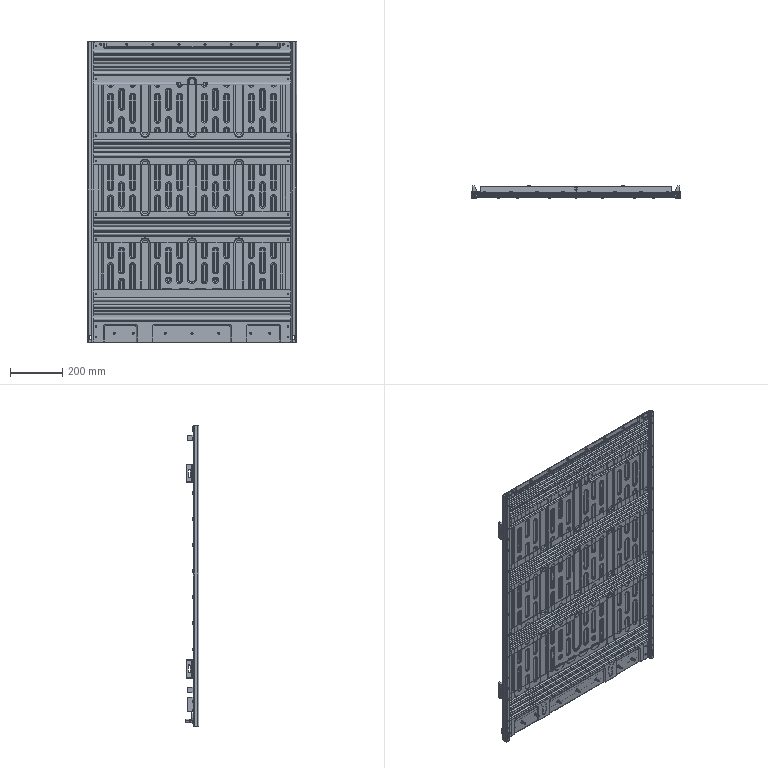Part | NX | features BREP 21 | 102 solids | 11159 faces | volume 4182433 mm3 | spline 3669 | cylinder 2703 | plane 2464 | torus 1631 | cone 398 | sphere 294 | commonest cylinder face diameters 1 x355 7 x355 5 x317 10 x195 9 x176 6 x160